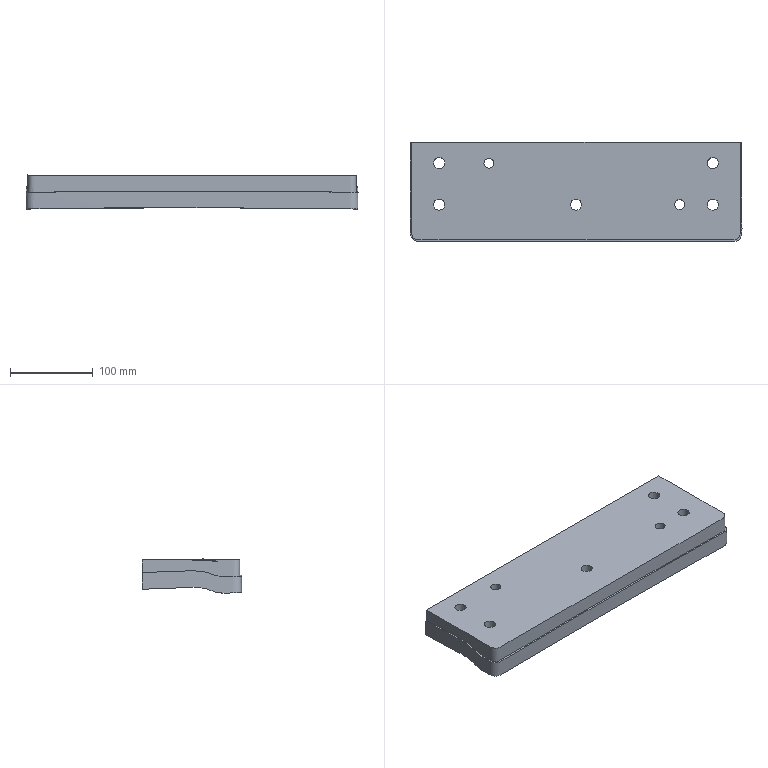Part | NX | features solid 2 | 1 solid | 36 faces | box 400.136 x 119.464 x 40.017 mm | volume 1469467 mm3 | cylinder 14 | spline 12 | plane 10 | commonest cylinder face diameters 13.5 x5 20 x5 12 x2 30 x2